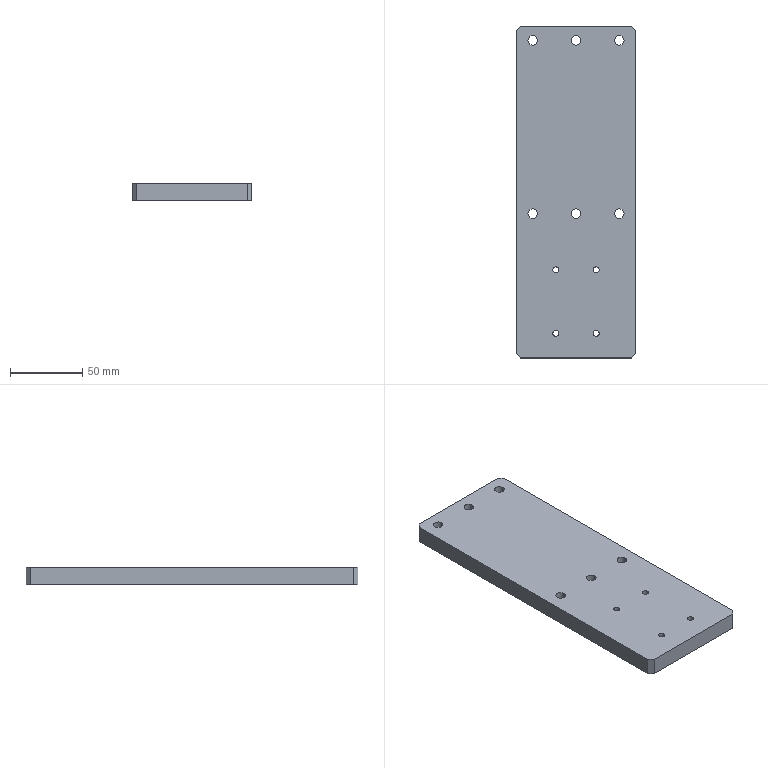Part | STEP file | 0-19-04 Lower cylinder mounting plate 1 | 1 solid | 48 faces | box 83 x 230 x 12 mm | volume 223254 mm3 | cylinder 32 | plane 16 | commonest cylinder face diameters 6.6 x12 11 x12 4.2 x8